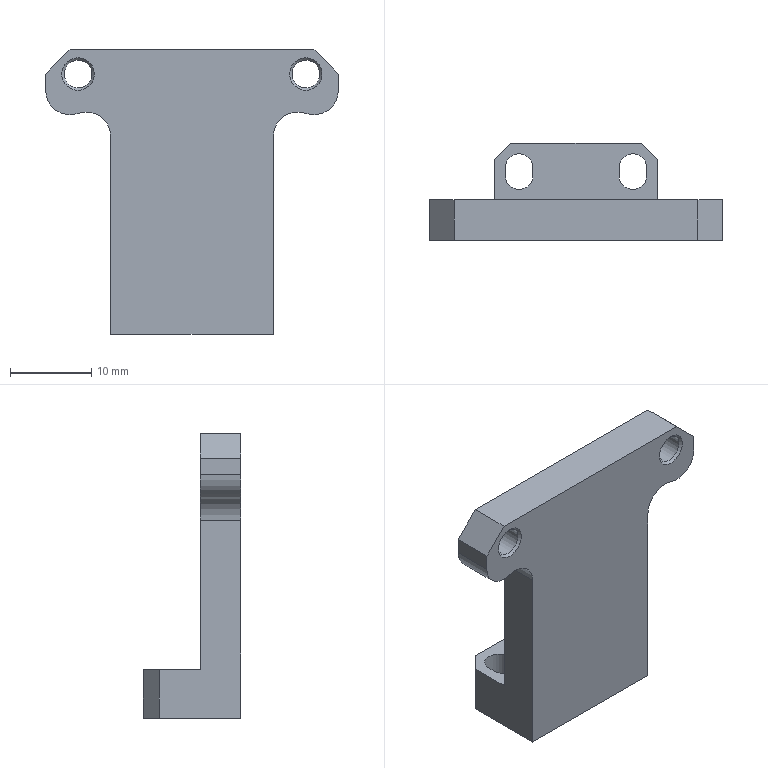Part | NX | features DATUM_CSYS 5, SKETCH 4, EXTRUDE 3, CHAMFER 2, OFFSET_REGION 2, SIMPLE HOLE 2, BLEND 1, HOLE PACKAGE 1 | 1 solid | 30 faces | box 36 x 12 x 35 mm | volume 4656 mm3 | plane 18 | cylinder 10 | cone 2 | commonest cylinder face diameters 3.4 x6 6 x4
STEP:
#1=CARTESIAN_POINT('',(23.3,9.,5.));
#2=VERTEX_POINT('',#1);
#3=CARTESIAN_POINT('',(23.3,8.,5.));
#4=VERTEX_POINT('',#3);
#5=CARTESIAN_POINT('',(23.3,9.,5.));
#6=DIRECTION('',(0.,-1.,0.));
#7=VECTOR('',#6,1000.);
#8=LINE('',#5,#7);
#9=EDGE_CURVE('',#2,#4,#8,.T.);
#10=ORIENTED_EDGE('',*,*,#9,.F.);
#11=CARTESIAN_POINT('',(26.7,9.,5.));
#12=VERTEX_POINT('',#11);
#13=CARTESIAN_POINT('',(25.,9.,5.));
#14=DIRECTION('',(0.,0.,1.));
#15=DIRECTION('',(0.,1.,0.));
#16=AXIS2_PLACEMENT_3D('',#13,#14,#15);
#17=CIRCLE('',#16,1.7);
#18=EDGE_CURVE('',#12,#2,#17,.T.);
#19=ORIENTED_EDGE('',*,*,#18,.F.);
#20=CARTESIAN_POINT('',(26.7,8.,5.));
#21=VERTEX_POINT('',#20);
#22=CARTESIAN_POINT('',(26.7,8.,5.));
#23=DIRECTION('',(0.,1.,0.));
#24=VECTOR('',#23,1000.);
#25=LINE('',#22,#24);
#26=EDGE_CURVE('',#21,#12,#25,.T.);
#27=ORIENTED_EDGE('',*,*,#26,.F.);
#28=CARTESIAN_POINT('',(25.,8.,5.));
#29=DIRECTION('',(0.,0.,1.));
#30=DIRECTION('',(0.,1.,0.));
#31=AXIS2_PLACEMENT_3D('',#28,#29,#30);
#32=CIRCLE('',#31,1.7);
#33=EDGE_CURVE('',#4,#21,#32,.T.);
#34=ORIENTED_EDGE('',*,*,#33,.F.);
#35=EDGE_LOOP('',(#10,#19,#27,#34));
#36=FACE_BOUND('',#35,.T.);
#37=CARTESIAN_POINT('',(26.,12.,5.));
#38=VERTEX_POINT('',#37);
#39=CARTESIAN_POINT('',(10.,12.,5.));
#40=VERTEX_POINT('',#39);
#41=CARTESIAN_POINT('',(36.,12.,5.));
#42=DIRECTION('',(-1.,0.,0.));
#43=VECTOR('',#42,1000.);
#44=LINE('',#41,#43);
#45=EDGE_CURVE('',#38,#40,#44,.T.);
#46=ORIENTED_EDGE('',*,*,#45,.T.);
#47=CARTESIAN_POINT('',(8.,10.,5.));
#48=VERTEX_POINT('',#47);
#49=CARTESIAN_POINT('',(8.,10.,5.));
#50=DIRECTION('',(0.7071,0.7071,0.));
#51=VECTOR('',#50,1000.);
#52=LINE('',#49,#51);
#53=EDGE_CURVE('',#40,#48,#52,.F.);
#54=ORIENTED_EDGE('',*,*,#53,.T.);
#55=CARTESIAN_POINT('',(8.,5.,5.));
#56=VERTEX_POINT('',#55);
#57=CARTESIAN_POINT('',(8.,12.,5.));
#58=DIRECTION('',(0.,-1.,0.));
#59=VECTOR('',#58,1000.);
#60=LINE('',#57,#59);
#61=EDGE_CURVE('',#48,#56,#60,.T.);
#62=ORIENTED_EDGE('',*,*,#61,.T.);
#63=CARTESIAN_POINT('',(28.,5.,5.));
#64=VERTEX_POINT('',#63);
#65=CARTESIAN_POINT('',(36.,5.,5.));
#66=DIRECTION('',(-1.,0.,0.));
#67=VECTOR('',#66,1000.);
#68=LINE('',#65,#67);
#69=EDGE_CURVE('',#64,#56,#68,.T.);
#70=ORIENTED_EDGE('',*,*,#69,.F.);
#71=CARTESIAN_POINT('',(28.,10.,5.));
#72=VERTEX_POINT('',#71);
#73=CARTESIAN_POINT('',(28.,12.,5.));
#74=DIRECTION('',(0.,1.,0.));
#75=VECTOR('',#74,1000.);
#76=LINE('',#73,#75);
#77=EDGE_CURVE('',#64,#72,#76,.T.);
#78=ORIENTED_EDGE('',*,*,#77,.T.);
#79=CARTESIAN_POINT('',(28.,10.,5.));
#80=DIRECTION('',(0.7071,-0.7071,0.));
#81=VECTOR('',#80,1000.);
#82=LINE('',#79,#81);
#83=EDGE_CURVE('',#72,#38,#82,.F.);
#84=ORIENTED_EDGE('',*,*,#83,.T.);
#85=EDGE_LOOP('',(#46,#54,#62,#70,#78,#84));
#86=FACE_BOUND('',#85,.T.);
#87=CARTESIAN_POINT('',(9.3,9.,5.));
#88=VERTEX_POINT('',#87);
#89=CARTESIAN_POINT('',(9.3,8.,5.));
#90=VERTEX_POINT('',#89);
#91=CARTESIAN_POINT('',(9.3,9.,5.));
#92=DIRECTION('',(0.,-1.,0.));
#93=VECTOR('',#92,1000.);
#94=LINE('',#91,#93);
#95=EDGE_CURVE('',#88,#90,#94,.T.);
#96=ORIENTED_EDGE('',*,*,#95,.F.);
#97=CARTESIAN_POINT('',(12.7,9.,5.));
#98=VERTEX_POINT('',#97);
#99=CARTESIAN_POINT('',(11.,9.,5.));
#100=DIRECTION('',(0.,0.,1.));
#101=DIRECTION('',(0.,1.,0.));
#102=AXIS2_PLACEMENT_3D('',#99,#100,#101);
#103=CIRCLE('',#102,1.7);
#104=EDGE_CURVE('',#98,#88,#103,.T.);
#105=ORIENTED_EDGE('',*,*,#104,.F.);
#106=CARTESIAN_POINT('',(12.7,8.,5.));
#107=VERTEX_POINT('',#106);
#108=CARTESIAN_POINT('',(12.7,8.,5.));
#109=DIRECTION('',(0.,1.,0.));
#110=VECTOR('',#109,1000.);
#111=LINE('',#108,#110);
#112=EDGE_CURVE('',#107,#98,#111,.T.);
#113=ORIENTED_EDGE('',*,*,#112,.F.);
#114=CARTESIAN_POINT('',(11.,8.,5.));
#115=DIRECTION('',(0.,0.,1.));
#116=DIRECTION('',(0.,1.,0.));
#117=AXIS2_PLACEMENT_3D('',#114,#115,#116);
#118=CIRCLE('',#117,1.7);
#119=EDGE_CURVE('',#90,#107,#118,.T.);
#120=ORIENTED_EDGE('',*,*,#119,.F.);
#121=EDGE_LOOP('',(#96,#105,#113,#120));
#122=FACE_BOUND('',#121,.T.);
#123=CARTESIAN_POINT('',(36.,12.,5.));
#124=DIRECTION('',(0.,0.,-1.));
#125=DIRECTION('',(0.,1.,0.));
#126=AXIS2_PLACEMENT_3D('',#123,#124,#125);
#127=PLANE('',#126);
#128=ADVANCED_FACE('',(#36,#86,#122),#127,.F.);
#129=CARTESIAN_POINT('',(26.,12.,-1.));
#130=VERTEX_POINT('',#129);
#131=CARTESIAN_POINT('',(10.,12.,-1.));
#132=VERTEX_POINT('',#131);
#133=CARTESIAN_POINT('',(36.,12.,-1.));
#134=DIRECTION('',(-1.,0.,0.));
#135=VECTOR('',#134,1000.);
#136=LINE('',#133,#135);
#137=EDGE_CURVE('',#130,#132,#136,.T.);
#138=ORIENTED_EDGE('',*,*,#137,.T.);
#139=CARTESIAN_POINT('',(10.,12.,0.));
#140=DIRECTION('',(0.,0.,1.));
#141=VECTOR('',#140,1000.);
#142=LINE('',#139,#141);
#143=EDGE_CURVE('',#132,#40,#142,.T.);
#144=ORIENTED_EDGE('',*,*,#143,.T.);
#145=ORIENTED_EDGE('',*,*,#45,.F.);
#146=CARTESIAN_POINT('',(26.,12.,0.));
#147=DIRECTION('',(0.,0.,-1.));
#148=VECTOR('',#147,1000.);
#149=LINE('',#146,#148);
#150=EDGE_CURVE('',#38,#130,#149,.T.);
#151=ORIENTED_EDGE('',*,*,#150,.T.);
#152=EDGE_LOOP('',(#138,#144,#145,#151));
#153=FACE_BOUND('',#152,.T.);
#154=CARTESIAN_POINT('',(36.,12.,0.));
#155=DIRECTION('',(0.,-1.,0.));
#156=DIRECTION('',(0.,0.,-1.));
#157=AXIS2_PLACEMENT_3D('',#154,#155,#156);
#158=PLANE('',#157);
#159=ADVANCED_FACE('',(#153),#158,.F.);
#160=CARTESIAN_POINT('',(0.,0.,31.));
#161=VERTEX_POINT('',#160);
#162=CARTESIAN_POINT('',(0.,0.,29.));
#163=VERTEX_POINT('',#162);
#164=CARTESIAN_POINT('',(0.,0.,34.));
#165=DIRECTION('',(0.,0.,-1.));
#166=VECTOR('',#165,1000.);
#167=LINE('',#164,#166);
#168=EDGE_CURVE('',#161,#163,#167,.T.);
#169=ORIENTED_EDGE('',*,*,#168,.F.);
#170=CARTESIAN_POINT('',(0.,5.,31.));
#171=VERTEX_POINT('',#170);
#172=CARTESIAN_POINT('',(0.,0.,31.));
#173=DIRECTION('',(0.,1.,0.));
#174=VECTOR('',#173,1000.);
#175=LINE('',#172,#174);
#176=EDGE_CURVE('',#161,#171,#175,.T.);
#177=ORIENTED_EDGE('',*,*,#176,.T.);
#178=CARTESIAN_POINT('',(0.,5.,29.));
#179=VERTEX_POINT('',#178);
#180=CARTESIAN_POINT('',(0.,5.,5.));
#181=DIRECTION('',(0.,0.,1.));
#182=VECTOR('',#181,1000.);
#183=LINE('',#180,#182);
#184=EDGE_CURVE('',#179,#171,#183,.T.);
#185=ORIENTED_EDGE('',*,*,#184,.F.);
#186=CARTESIAN_POINT('',(0.,0.,29.));
#187=DIRECTION('',(0.,1.,0.));
#188=VECTOR('',#187,1000.);
#189=LINE('',#186,#188);
#190=EDGE_CURVE('',#179,#163,#189,.F.);
#191=ORIENTED_EDGE('',*,*,#190,.T.);
#192=EDGE_LOOP('',(#169,#177,#185,#191));
#193=FACE_BOUND('',#192,.T.);
#194=CARTESIAN_POINT('',(0.,0.,0.));
#195=DIRECTION('',(1.,0.,0.));
#196=DIRECTION('',(0.,0.,-1.));
#197=AXIS2_PLACEMENT_3D('',#194,#195,#196);
#198=PLANE('',#197);
#199=ADVANCED_FACE('',(#193),#198,.F.);
#200=CARTESIAN_POINT('',(12.7,9.,-1.));
#201=VERTEX_POINT('',#200);
#202=CARTESIAN_POINT('',(9.3,9.,-1.));
#203=VERTEX_POINT('',#202);
#204=CARTESIAN_POINT('',(11.,9.,-1.));
#205=DIRECTION('',(0.,0.,1.));
#206=DIRECTION('',(1.,0.,0.));
#207=AXIS2_PLACEMENT_3D('',#204,#205,#206);
#208=CIRCLE('',#207,1.7);
#209=EDGE_CURVE('',#201,#203,#208,.T.);
#210=ORIENTED_EDGE('',*,*,#209,.T.);
#211=CARTESIAN_POINT('',(9.3,8.,-1.));
#212=VERTEX_POINT('',#211);
#213=CARTESIAN_POINT('',(9.3,5.,-1.));
#214=DIRECTION('',(0.,-1.,0.));
#215=VECTOR('',#214,1000.);
#216=LINE('',#213,#215);
#217=EDGE_CURVE('',#203,#212,#216,.T.);
#218=ORIENTED_EDGE('',*,*,#217,.T.);
#219=CARTESIAN_POINT('',(12.7,8.,-1.));
#220=VERTEX_POINT('',#219);
#221=CARTESIAN_POINT('',(11.,8.,-1.));
#222=DIRECTION('',(0.,0.,1.));
#223=DIRECTION('',(1.,0.,0.));
#224=AXIS2_PLACEMENT_3D('',#221,#222,#223);
#225=CIRCLE('',#224,1.7);
#226=EDGE_CURVE('',#212,#220,#225,.T.);
#227=ORIENTED_EDGE('',*,*,#226,.T.);
#228=CARTESIAN_POINT('',(12.7,5.,-1.));
#229=DIRECTION('',(0.,1.,0.));
#230=VECTOR('',#229,1000.);
#231=LINE('',#228,#230);
#232=EDGE_CURVE('',#220,#201,#231,.T.);
#233=ORIENTED_EDGE('',*,*,#232,.T.);
#234=EDGE_LOOP('',(#210,#218,#227,#233));
#235=FACE_BOUND('',#234,.T.);
#236=CARTESIAN_POINT('',(26.7,9.,-1.));
#237=VERTEX_POINT('',#236);
#238=CARTESIAN_POINT('',(23.3,9.,-1.));
#239=VERTEX_POINT('',#238);
#240=CARTESIAN_POINT('',(25.,9.,-1.));
#241=DIRECTION('',(0.,0.,1.));
#242=DIRECTION('',(1.,0.,0.));
#243=AXIS2_PLACEMENT_3D('',#240,#241,#242);
#244=CIRCLE('',#243,1.7);
#245=EDGE_CURVE('',#237,#239,#244,.T.);
#246=ORIENTED_EDGE('',*,*,#245,.T.);
#247=CARTESIAN_POINT('',(23.3,8.,-1.));
#248=VERTEX_POINT('',#247);
#249=CARTESIAN_POINT('',(23.3,5.,-1.));
#250=DIRECTION('',(0.,-1.,0.));
#251=VECTOR('',#250,1000.);
#252=LINE('',#249,#251);
#253=EDGE_CURVE('',#239,#248,#252,.T.);
#254=ORIENTED_EDGE('',*,*,#253,.T.);
#255=CARTESIAN_POINT('',(26.7,8.,-1.));
#256=VERTEX_POINT('',#255);
#257=CARTESIAN_POINT('',(25.,8.,-1.));
#258=DIRECTION('',(0.,0.,1.));
#259=DIRECTION('',(1.,0.,0.));
#260=AXIS2_PLACEMENT_3D('',#257,#258,#259);
#261=CIRCLE('',#260,1.7);
#262=EDGE_CURVE('',#248,#256,#261,.T.);
#263=ORIENTED_EDGE('',*,*,#262,.T.);
#264=CARTESIAN_POINT('',(26.7,5.,-1.));
#265=DIRECTION('',(0.,1.,0.));
#266=VECTOR('',#265,1000.);
#267=LINE('',#264,#266);
#268=EDGE_CURVE('',#256,#237,#267,.T.);
#269=ORIENTED_EDGE('',*,*,#268,.T.);
#270=EDGE_LOOP('',(#246,#254,#263,#269));
#271=FACE_BOUND('',#270,.T.);
#272=CARTESIAN_POINT('',(8.,0.,-1.));
#273=VERTEX_POINT('',#272);
#274=CARTESIAN_POINT('',(8.,10.,-1.));
#275=VERTEX_POINT('',#274);
#276=CARTESIAN_POINT('',(8.,5.,-1.));
#277=DIRECTION('',(0.,1.,0.));
#278=VECTOR('',#277,1000.);
#279=LINE('',#276,#278);
#280=EDGE_CURVE('',#273,#275,#279,.T.);
#281=ORIENTED_EDGE('',*,*,#280,.T.);
#282=CARTESIAN_POINT('',(8.,10.,-1.));
#283=DIRECTION('',(-0.7071,-0.7071,0.));
#284=VECTOR('',#283,1000.);
#285=LINE('',#282,#284);
#286=EDGE_CURVE('',#275,#132,#285,.F.);
#287=ORIENTED_EDGE('',*,*,#286,.T.);
#288=ORIENTED_EDGE('',*,*,#137,.F.);
#289=CARTESIAN_POINT('',(28.,10.,-1.));
#290=VERTEX_POINT('',#289);
#291=CARTESIAN_POINT('',(28.,10.,-1.));
#292=DIRECTION('',(-0.7071,0.7071,0.));
#293=VECTOR('',#292,1000.);
#294=LINE('',#291,#293);
#295=EDGE_CURVE('',#130,#290,#294,.F.);
#296=ORIENTED_EDGE('',*,*,#295,.T.);
#297=CARTESIAN_POINT('',(28.,0.,-1.));
#298=VERTEX_POINT('',#297);
#299=CARTESIAN_POINT('',(28.,-38.,-1.));
#300=DIRECTION('',(0.,1.,0.));
#301=VECTOR('',#300,1000.);
#302=LINE('',#299,#301);
#303=EDGE_CURVE('',#298,#290,#302,.T.);
#304=ORIENTED_EDGE('',*,*,#303,.F.);
#305=CARTESIAN_POINT('',(36.,0.,-1.));
#306=DIRECTION('',(-1.,0.,0.));
#307=VECTOR('',#306,1000.);
#308=LINE('',#305,#307);
#309=EDGE_CURVE('',#298,#273,#308,.T.);
#310=ORIENTED_EDGE('',*,*,#309,.T.);
#311=EDGE_LOOP('',(#281,#287,#288,#296,#304,#310));
#312=FACE_BOUND('',#311,.T.);
#313=CARTESIAN_POINT('',(36.,5.,-1.));
#314=DIRECTION('',(0.,0.,1.));
#315=DIRECTION('',(1.,0.,0.));
#316=AXIS2_PLACEMENT_3D('',#313,#314,#315);
#317=PLANE('',#316);
#318=ADVANCED_FACE('',(#235,#271,#312),#317,.F.);
#319=CARTESIAN_POINT('',(36.,5.,29.));
#320=VERTEX_POINT('',#319);
#321=CARTESIAN_POINT('',(36.,5.,31.));
#322=VERTEX_POINT('',#321);
#323=CARTESIAN_POINT('',(36.,5.,5.));
#324=DIRECTION('',(0.,0.,1.));
#325=VECTOR('',#324,1000.);
#326=LINE('',#323,#325);
#327=EDGE_CURVE('',#320,#322,#326,.T.);
#328=ORIENTED_EDGE('',*,*,#327,.T.);
#329=CARTESIAN_POINT('',(36.,0.,31.));
#330=VERTEX_POINT('',#329);
#331=CARTESIAN_POINT('',(36.,0.,31.));
#332=DIRECTION('',(0.,-1.,0.));
#333=VECTOR('',#332,1000.);
#334=LINE('',#331,#333);
#335=EDGE_CURVE('',#322,#330,#334,.T.);
#336=ORIENTED_EDGE('',*,*,#335,.T.);
#337=CARTESIAN_POINT('',(36.,0.,29.));
#338=VERTEX_POINT('',#337);
#339=CARTESIAN_POINT('',(36.,0.,5.));
#340=DIRECTION('',(0.,0.,-1.));
#341=VECTOR('',#340,1000.);
#342=LINE('',#339,#341);
#343=EDGE_CURVE('',#330,#338,#342,.T.);
#344=ORIENTED_EDGE('',*,*,#343,.T.);
#345=CARTESIAN_POINT('',(36.,5.,29.));
#346=DIRECTION('',(0.,1.,0.));
#347=VECTOR('',#346,1000.);
#348=LINE('',#345,#347);
#349=EDGE_CURVE('',#338,#320,#348,.T.);
#350=ORIENTED_EDGE('',*,*,#349,.T.);
#351=EDGE_LOOP('',(#328,#336,#344,#350));
#352=FACE_BOUND('',#351,.T.);
#353=CARTESIAN_POINT('',(36.,0.,0.));
#354=DIRECTION('',(1.,0.,0.));
#355=DIRECTION('',(0.,0.,-1.));
#356=AXIS2_PLACEMENT_3D('',#353,#354,#355);
#357=PLANE('',#356);
#358=ADVANCED_FACE('',(#352),#357,.T.);
#359=CARTESIAN_POINT('',(3.995,5.,29.3));
#360=VERTEX_POINT('',#359);
#361=CARTESIAN_POINT('',(3.995,5.,31.));
#362=DIRECTION('',(0.,-1.,0.));
#363=DIRECTION('',(0.,0.,-1.));
#364=AXIS2_PLACEMENT_3D('',#361,#362,#363);
#365=CIRCLE('',#364,1.7);
#366=EDGE_CURVE('',#360,#360,#365,.T.);
#367=ORIENTED_EDGE('',*,*,#366,.T.);
#368=EDGE_LOOP('',(#367));
#369=FACE_BOUND('',#368,.T.);
#370=CARTESIAN_POINT('',(32.,5.,29.3));
#371=VERTEX_POINT('',#370);
#372=CARTESIAN_POINT('',(32.,5.,31.));
#373=DIRECTION('',(0.,-1.,0.));
#374=DIRECTION('',(0.,0.,-1.));
#375=AXIS2_PLACEMENT_3D('',#372,#373,#374);
#376=CIRCLE('',#375,1.7);
#377=EDGE_CURVE('',#371,#371,#376,.T.);
#378=ORIENTED_EDGE('',*,*,#377,.T.);
#379=EDGE_LOOP('',(#378));
#380=FACE_BOUND('',#379,.T.);
#381=CARTESIAN_POINT('',(33.,5.,34.));
#382=VERTEX_POINT('',#381);
#383=CARTESIAN_POINT('',(3.,5.,34.));
#384=VERTEX_POINT('',#383);
#385=CARTESIAN_POINT('',(36.,5.,34.));
#386=DIRECTION('',(-1.,0.,0.));
#387=VECTOR('',#386,1000.);
#388=LINE('',#385,#387);
#389=EDGE_CURVE('',#382,#384,#388,.T.);
#390=ORIENTED_EDGE('',*,*,#389,.F.);
#391=CARTESIAN_POINT('',(36.,5.,31.));
#392=DIRECTION('',(0.7071,0.,-0.7071));
#393=VECTOR('',#392,1000.);
#394=LINE('',#391,#393);
#395=EDGE_CURVE('',#382,#322,#394,.T.);
#396=ORIENTED_EDGE('',*,*,#395,.T.);
#397=ORIENTED_EDGE('',*,*,#327,.F.);
#398=CARTESIAN_POINT('',(32.,5.,26.172));
#399=VERTEX_POINT('',#398);
#400=CARTESIAN_POINT('',(33.,5.,29.));
#401=DIRECTION('',(0.,-1.,0.));
#402=DIRECTION('',(0.,0.,-1.));
#403=AXIS2_PLACEMENT_3D('',#400,#401,#402);
#404=CIRCLE('',#403,3.);
#405=EDGE_CURVE('',#320,#399,#404,.F.);
#406=ORIENTED_EDGE('',*,*,#405,.T.);
#407=CARTESIAN_POINT('',(28.,5.,23.343));
#408=VERTEX_POINT('',#407);
#409=CARTESIAN_POINT('',(31.,5.,23.343));
#410=DIRECTION('',(0.,-1.,0.));
#411=DIRECTION('',(0.,0.,-1.));
#412=AXIS2_PLACEMENT_3D('',#409,#410,#411);
#413=CIRCLE('',#412,3.);
#414=EDGE_CURVE('',#399,#408,#413,.T.);
#415=ORIENTED_EDGE('',*,*,#414,.T.);
#416=CARTESIAN_POINT('',(28.,5.,5.));
#417=DIRECTION('',(0.,0.,-1.));
#418=VECTOR('',#417,1000.);
#419=LINE('',#416,#418);
#420=EDGE_CURVE('',#408,#64,#419,.T.);
#421=ORIENTED_EDGE('',*,*,#420,.T.);
#422=ORIENTED_EDGE('',*,*,#69,.T.);
#423=CARTESIAN_POINT('',(8.,5.,23.343));
#424=VERTEX_POINT('',#423);
#425=CARTESIAN_POINT('',(8.,5.,5.));
#426=DIRECTION('',(0.,0.,1.));
#427=VECTOR('',#426,1000.);
#428=LINE('',#425,#427);
#429=EDGE_CURVE('',#56,#424,#428,.T.);
#430=ORIENTED_EDGE('',*,*,#429,.T.);
#431=CARTESIAN_POINT('',(4.,5.,26.172));
#432=VERTEX_POINT('',#431);
#433=CARTESIAN_POINT('',(5.,5.,23.343));
#434=DIRECTION('',(0.,-1.,0.));
#435=DIRECTION('',(0.,0.,-1.));
#436=AXIS2_PLACEMENT_3D('',#433,#434,#435);
#437=CIRCLE('',#436,3.);
#438=EDGE_CURVE('',#424,#432,#437,.T.);
#439=ORIENTED_EDGE('',*,*,#438,.T.);
#440=CARTESIAN_POINT('',(3.,5.,29.));
#441=DIRECTION('',(0.,-1.,0.));
#442=DIRECTION('',(0.,0.,-1.));
#443=AXIS2_PLACEMENT_3D('',#440,#441,#442);
#444=CIRCLE('',#443,3.);
#445=EDGE_CURVE('',#432,#179,#444,.F.);
#446=ORIENTED_EDGE('',*,*,#445,.T.);
#447=ORIENTED_EDGE('',*,*,#184,.T.);
#448=CARTESIAN_POINT('',(3.,5.,34.));
#449=DIRECTION('',(-0.7071,0.,-0.7071));
#450=VECTOR('',#449,1000.);
#451=LINE('',#448,#450);
#452=EDGE_CURVE('',#171,#384,#451,.F.);
#453=ORIENTED_EDGE('',*,*,#452,.T.);
#454=EDGE_LOOP('',(#390,#396,#397,#406,#415,#421,#422,#430,#439,#446,#447,#453));
#455=FACE_BOUND('',#454,.T.);
#456=CARTESIAN_POINT('',(36.,5.,5.));
#457=DIRECTION('',(0.,-1.,0.));
#458=DIRECTION('',(0.,0.,-1.));
#459=AXIS2_PLACEMENT_3D('',#456,#457,#458);
#460=PLANE('',#459);
#461=ADVANCED_FACE('',(#369,#380,#455),#460,.F.);
#462=CARTESIAN_POINT('',(33.,0.,34.));
#463=VERTEX_POINT('',#462);
#464=CARTESIAN_POINT('',(3.,0.,34.));
#465=VERTEX_POINT('',#464);
#466=CARTESIAN_POINT('',(36.,0.,34.));
#467=DIRECTION('',(-1.,0.,0.));
#468=VECTOR('',#467,1000.);
#469=LINE('',#466,#468);
#470=EDGE_CURVE('',#463,#465,#469,.T.);
#471=ORIENTED_EDGE('',*,*,#470,.F.);
#472=CARTESIAN_POINT('',(33.,5.,34.));
#473=DIRECTION('',(0.,1.,0.));
#474=VECTOR('',#473,1000.);
#475=LINE('',#472,#474);
#476=EDGE_CURVE('',#463,#382,#475,.T.);
#477=ORIENTED_EDGE('',*,*,#476,.T.);
#478=ORIENTED_EDGE('',*,*,#389,.T.);
#479=CARTESIAN_POINT('',(3.,5.,34.));
#480=DIRECTION('',(0.,-1.,0.));
#481=VECTOR('',#480,1000.);
#482=LINE('',#479,#481);
#483=EDGE_CURVE('',#384,#465,#482,.T.);
#484=ORIENTED_EDGE('',*,*,#483,.T.);
#485=EDGE_LOOP('',(#471,#477,#478,#484));
#486=FACE_BOUND('',#485,.T.);
#487=CARTESIAN_POINT('',(36.,5.,34.));
#488=DIRECTION('',(0.,0.,-1.));
#489=DIRECTION('',(-1.,0.,0.));
#490=AXIS2_PLACEMENT_3D('',#487,#488,#489);
#491=PLANE('',#490);
#492=ADVANCED_FACE('',(#486),#491,.F.);
#493=CARTESIAN_POINT('',(3.995,0.,33.));
#494=VERTEX_POINT('',#493);
#495=CARTESIAN_POINT('',(3.995,0.,31.));
#496=DIRECTION('',(0.,1.,0.));
#497=DIRECTION('',(0.,0.,1.));
#498=AXIS2_PLACEMENT_3D('',#495,#496,#497);
#499=CIRCLE('',#498,2.);
#500=EDGE_CURVE('',#494,#494,#499,.T.);
#501=ORIENTED_EDGE('',*,*,#500,.T.);
#502=EDGE_LOOP('',(#501));
#503=FACE_BOUND('',#502,.T.);
#504=CARTESIAN_POINT('',(32.,0.,33.));
#505=VERTEX_POINT('',#504);
#506=CARTESIAN_POINT('',(32.,0.,31.));
#507=DIRECTION('',(0.,1.,0.));
#508=DIRECTION('',(0.,0.,1.));
#509=AXIS2_PLACEMENT_3D('',#506,#507,#508);
#510=CIRCLE('',#509,2.);
#511=EDGE_CURVE('',#505,#505,#510,.T.);
#512=ORIENTED_EDGE('',*,*,#511,.T.);
#513=EDGE_LOOP('',(#512));
#514=FACE_BOUND('',#513,.T.);
#515=ORIENTED_EDGE('',*,*,#343,.F.);
#516=CARTESIAN_POINT('',(36.,0.,31.));
#517=DIRECTION('',(-0.7071,0.,0.7071));
#518=VECTOR('',#517,1000.);
#519=LINE('',#516,#518);
#520=EDGE_CURVE('',#330,#463,#519,.T.);
#521=ORIENTED_EDGE('',*,*,#520,.T.);
#522=ORIENTED_EDGE('',*,*,#470,.T.);
#523=CARTESIAN_POINT('',(3.,0.,34.));
#524=DIRECTION('',(0.7071,0.,0.7071));
#525=VECTOR('',#524,1000.);
#526=LINE('',#523,#525);
#527=EDGE_CURVE('',#465,#161,#526,.F.);
#528=ORIENTED_EDGE('',*,*,#527,.T.);
#529=ORIENTED_EDGE('',*,*,#168,.T.);
#530=CARTESIAN_POINT('',(4.,0.,26.172));
#531=VERTEX_POINT('',#530);
#532=CARTESIAN_POINT('',(3.,0.,29.));
#533=DIRECTION('',(0.,1.,0.));
#534=DIRECTION('',(0.,0.,1.));
#535=AXIS2_PLACEMENT_3D('',#532,#533,#534);
#536=CIRCLE('',#535,3.);
#537=EDGE_CURVE('',#163,#531,#536,.F.);
#538=ORIENTED_EDGE('',*,*,#537,.T.);
#539=CARTESIAN_POINT('',(8.,0.,23.343));
#540=VERTEX_POINT('',#539);
#541=CARTESIAN_POINT('',(5.,0.,23.343));
#542=DIRECTION('',(0.,1.,0.));
#543=DIRECTION('',(0.,0.,1.));
#544=AXIS2_PLACEMENT_3D('',#541,#542,#543);
#545=CIRCLE('',#544,3.);
#546=EDGE_CURVE('',#531,#540,#545,.T.);
#547=ORIENTED_EDGE('',*,*,#546,.T.);
#548=CARTESIAN_POINT('',(8.,0.,34.));
#549=DIRECTION('',(0.,0.,-1.));
#550=VECTOR('',#549,1000.);
#551=LINE('',#548,#550);
#552=EDGE_CURVE('',#540,#273,#551,.T.);
#553=ORIENTED_EDGE('',*,*,#552,.T.);
#554=ORIENTED_EDGE('',*,*,#309,.F.);
#555=CARTESIAN_POINT('',(28.,0.,23.343));
#556=VERTEX_POINT('',#555);
#557=CARTESIAN_POINT('',(28.,0.,34.));
#558=DIRECTION('',(0.,0.,1.));
#559=VECTOR('',#558,1000.);
#560=LINE('',#557,#559);
#561=EDGE_CURVE('',#298,#556,#560,.T.);
#562=ORIENTED_EDGE('',*,*,#561,.T.);
#563=CARTESIAN_POINT('',(32.,0.,26.172));
#564=VERTEX_POINT('',#563);
#565=CARTESIAN_POINT('',(31.,0.,23.343));
#566=DIRECTION('',(0.,1.,0.));
#567=DIRECTION('',(0.,0.,1.));
#568=AXIS2_PLACEMENT_3D('',#565,#566,#567);
#569=CIRCLE('',#568,3.);
#570=EDGE_CURVE('',#556,#564,#569,.T.);
#571=ORIENTED_EDGE('',*,*,#570,.T.);
#572=CARTESIAN_POINT('',(33.,0.,29.));
#573=DIRECTION('',(0.,1.,0.));
#574=DIRECTION('',(0.,0.,1.));
#575=AXIS2_PLACEMENT_3D('',#572,#573,#574);
#576=CIRCLE('',#575,3.);
#577=EDGE_CURVE('',#564,#338,#576,.F.);
#578=ORIENTED_EDGE('',*,*,#577,.T.);
#579=EDGE_LOOP('',(#515,#521,#522,#528,#529,#538,#547,#553,#554,#562,#571,#578));
#580=FACE_BOUND('',#579,.T.);
#581=CARTESIAN_POINT('',(36.,0.,34.));
#582=DIRECTION('',(0.,1.,0.));
#583=DIRECTION('',(0.,0.,1.));
#584=AXIS2_PLACEMENT_3D('',#581,#582,#583);
#585=PLANE('',#584);
#586=ADVANCED_FACE('',(#503,#514,#580),#585,.F.);
#587=CARTESIAN_POINT('',(32.,0.3,32.7));
#588=VERTEX_POINT('',#587);
#589=CARTESIAN_POINT('',(32.,0.3,31.));
#590=DIRECTION('',(0.,1.,0.));
#591=DIRECTION('',(0.,0.,1.));
#592=AXIS2_PLACEMENT_3D('',#589,#590,#591);
#593=CIRCLE('',#592,1.7);
#594=EDGE_CURVE('',#588,#588,#593,.F.);
#595=ORIENTED_EDGE('',*,*,#594,.T.);
#596=EDGE_LOOP('',(#595));
#597=FACE_BOUND('',#596,.T.);
#598=ORIENTED_EDGE('',*,*,#377,.F.);
#599=EDGE_LOOP('',(#598));
#600=FACE_BOUND('',#599,.T.);
#601=CARTESIAN_POINT('',(32.,5.,31.));
#602=DIRECTION('',(0.,-1.,0.));
#603=DIRECTION('',(0.,0.,-1.));
#604=AXIS2_PLACEMENT_3D('',#601,#602,#603);
#605=CYLINDRICAL_SURFACE('',#604,1.7);
#606=ADVANCED_FACE('',(#597,#600),#605,.F.);
#607=ORIENTED_EDGE('',*,*,#594,.F.);
#608=EDGE_LOOP('',(#607));
#609=FACE_BOUND('',#608,.T.);
#610=ORIENTED_EDGE('',*,*,#511,.F.);
#611=EDGE_LOOP('',(#610));
#612=FACE_BOUND('',#611,.T.);
#613=CARTESIAN_POINT('',(32.,0.,31.));
#614=DIRECTION('',(0.,-1.,0.));
#615=DIRECTION('',(0.,0.,-1.));
#616=AXIS2_PLACEMENT_3D('',#613,#614,#615);
#617=CONICAL_SURFACE('',#616,2.,0.7854);
#618=ADVANCED_FACE('',(#609,#612),#617,.F.);
#619=CARTESIAN_POINT('',(3.995,0.3,32.7));
#620=VERTEX_POINT('',#619);
#621=CARTESIAN_POINT('',(3.995,0.3,31.));
#622=DIRECTION('',(0.,1.,0.));
#623=DIRECTION('',(0.,0.,1.));
#624=AXIS2_PLACEMENT_3D('',#621,#622,#623);
#625=CIRCLE('',#624,1.7);
#626=EDGE_CURVE('',#620,#620,#625,.F.);
#627=ORIENTED_EDGE('',*,*,#626,.T.);
#628=EDGE_LOOP('',(#627));
#629=FACE_BOUND('',#628,.T.);
#630=ORIENTED_EDGE('',*,*,#366,.F.);
#631=EDGE_LOOP('',(#630));
#632=FACE_BOUND('',#631,.T.);
#633=CARTESIAN_POINT('',(3.995,5.,31.));
#634=DIRECTION('',(0.,-1.,0.));
#635=DIRECTION('',(0.,0.,-1.));
#636=AXIS2_PLACEMENT_3D('',#633,#634,#635);
#637=CYLINDRICAL_SURFACE('',#636,1.7);
#638=ADVANCED_FACE('',(#629,#632),#637,.F.);
#639=ORIENTED_EDGE('',*,*,#626,.F.);
#640=EDGE_LOOP('',(#639));
#641=FACE_BOUND('',#640,.T.);
#642=ORIENTED_EDGE('',*,*,#500,.F.);
#643=EDGE_LOOP('',(#642));
#644=FACE_BOUND('',#643,.T.);
#645=CARTESIAN_POINT('',(3.995,0.,31.));
#646=DIRECTION('',(0.,-1.,0.));
#647=DIRECTION('',(0.,0.,-1.));
#648=AXIS2_PLACEMENT_3D('',#645,#646,#647);
#649=CONICAL_SURFACE('',#648,2.,0.7854);
#650=ADVANCED_FACE('',(#641,#644),#649,.F.);
#651=ORIENTED_EDGE('',*,*,#303,.T.);
#652=CARTESIAN_POINT('',(28.,10.,-1.));
#653=DIRECTION('',(0.,0.,1.));
#654=VECTOR('',#653,1000.);
#655=LINE('',#652,#654);
#656=EDGE_CURVE('',#290,#72,#655,.T.);
#657=ORIENTED_EDGE('',*,*,#656,.T.);
#658=ORIENTED_EDGE('',*,*,#77,.F.);
#659=ORIENTED_EDGE('',*,*,#420,.F.);
#660=CARTESIAN_POINT('',(28.,2.5,23.343));
#661=DIRECTION('',(0.,1.,0.));
#662=VECTOR('',#661,1000.);
#663=LINE('',#660,#662);
#664=EDGE_CURVE('',#408,#556,#663,.F.);
#665=ORIENTED_EDGE('',*,*,#664,.T.);
#666=ORIENTED_EDGE('',*,*,#561,.F.);
#667=EDGE_LOOP('',(#651,#657,#658,#659,#665,#666));
#668=FACE_BOUND('',#667,.T.);
#669=CARTESIAN_POINT('',(28.,-38.,-1.));
#670=DIRECTION('',(-1.,0.,0.));
#671=DIRECTION('',(0.,0.,1.));
#672=AXIS2_PLACEMENT_3D('',#669,#670,#671);
#673=PLANE('',#672);
#674=ADVANCED_FACE('',(#668),#673,.F.);
#675=ORIENTED_EDGE('',*,*,#61,.F.);
#676=CARTESIAN_POINT('',(8.,10.,26.));
#677=DIRECTION('',(0.,0.,-1.));
#678=VECTOR('',#677,1000.);
#679=LINE('',#676,#678);
#680=EDGE_CURVE('',#48,#275,#679,.T.);
#681=ORIENTED_EDGE('',*,*,#680,.T.);
#682=ORIENTED_EDGE('',*,*,#280,.F.);
#683=ORIENTED_EDGE('',*,*,#552,.F.);
#684=CARTESIAN_POINT('',(8.,2.5,23.343));
#685=DIRECTION('',(0.,1.,0.));
#686=VECTOR('',#685,1000.);
#687=LINE('',#684,#686);
#688=EDGE_CURVE('',#540,#424,#687,.T.);
#689=ORIENTED_EDGE('',*,*,#688,.T.);
#690=ORIENTED_EDGE('',*,*,#429,.F.);
#691=EDGE_LOOP('',(#675,#681,#682,#683,#689,#690));
#692=FACE_BOUND('',#691,.T.);
#693=CARTESIAN_POINT('',(8.,-38.,26.));
#694=DIRECTION('',(1.,0.,0.));
#695=DIRECTION('',(0.,0.,-1.));
#696=AXIS2_PLACEMENT_3D('',#693,#694,#695);
#697=PLANE('',#696);
#698=ADVANCED_FACE('',(#692),#697,.F.);
#699=ORIENTED_EDGE('',*,*,#688,.F.);
#700=ORIENTED_EDGE('',*,*,#546,.F.);
#701=CARTESIAN_POINT('',(4.,2.5,26.172));
#702=DIRECTION('',(0.,1.,0.));
#703=VECTOR('',#702,1000.);
#704=LINE('',#701,#703);
#705=EDGE_CURVE('',#432,#531,#704,.F.);
#706=ORIENTED_EDGE('',*,*,#705,.F.);
#707=ORIENTED_EDGE('',*,*,#438,.F.);
#708=EDGE_LOOP('',(#699,#700,#706,#707));
#709=FACE_BOUND('',#708,.T.);
#710=CARTESIAN_POINT('',(5.,-38.,23.343));
#711=DIRECTION('',(0.,1.,0.));
#712=DIRECTION('',(0.,0.,1.));
#713=AXIS2_PLACEMENT_3D('',#710,#711,#712);
#714=CYLINDRICAL_SURFACE('',#713,3.);
#715=ADVANCED_FACE('',(#709),#714,.F.);
#716=ORIENTED_EDGE('',*,*,#537,.F.);
#717=ORIENTED_EDGE('',*,*,#190,.F.);
#718=ORIENTED_EDGE('',*,*,#445,.F.);
#719=ORIENTED_EDGE('',*,*,#705,.T.);
#720=EDGE_LOOP('',(#716,#717,#718,#719));
#721=FACE_BOUND('',#720,.T.);
#722=CARTESIAN_POINT('',(3.,-38.,29.));
#723=DIRECTION('',(0.,1.,0.));
#724=DIRECTION('',(0.,0.,1.));
#725=AXIS2_PLACEMENT_3D('',#722,#723,#724);
#726=CYLINDRICAL_SURFACE('',#725,3.);
#727=ADVANCED_FACE('',(#721),#726,.T.);
#728=CARTESIAN_POINT('',(32.,2.5,26.172));
#729=DIRECTION('',(0.,1.,0.));
#730=VECTOR('',#729,1000.);
#731=LINE('',#728,#730);
#732=EDGE_CURVE('',#399,#564,#731,.F.);
#733=ORIENTED_EDGE('',*,*,#732,.F.);
#734=ORIENTED_EDGE('',*,*,#405,.F.);
#735=ORIENTED_EDGE('',*,*,#349,.F.);
#736=ORIENTED_EDGE('',*,*,#577,.F.);
#737=EDGE_LOOP('',(#733,#734,#735,#736));
#738=FACE_BOUND('',#737,.T.);
#739=CARTESIAN_POINT('',(33.,0.,29.));
#740=DIRECTION('',(0.,-1.,0.));
#741=DIRECTION('',(0.,0.,-1.));
#742=AXIS2_PLACEMENT_3D('',#739,#740,#741);
#743=CYLINDRICAL_SURFACE('',#742,3.);
#744=ADVANCED_FACE('',(#738),#743,.T.);
#745=ORIENTED_EDGE('',*,*,#414,.F.);
#746=ORIENTED_EDGE('',*,*,#732,.T.);
#747=ORIENTED_EDGE('',*,*,#570,.F.);
#748=ORIENTED_EDGE('',*,*,#664,.F.);
#749=EDGE_LOOP('',(#745,#746,#747,#748));
#750=FACE_BOUND('',#749,.T.);
#751=CARTESIAN_POINT('',(31.,-38.,23.343));
#752=DIRECTION('',(0.,1.,0.));
#753=DIRECTION('',(0.,0.,1.));
#754=AXIS2_PLACEMENT_3D('',#751,#752,#753);
#755=CYLINDRICAL_SURFACE('',#754,3.);
#756=ADVANCED_FACE('',(#750),#755,.F.);
#757=CARTESIAN_POINT('',(23.3,9.,-45.));
#758=DIRECTION('',(0.,0.,1.));
#759=VECTOR('',#758,1000.);
#760=LINE('',#757,#759);
#761=EDGE_CURVE('',#2,#239,#760,.F.);
#762=ORIENTED_EDGE('',*,*,#761,.F.);
#763=ORIENTED_EDGE('',*,*,#9,.T.);
#764=CARTESIAN_POINT('',(23.3,8.,-45.));
#765=DIRECTION('',(0.,0.,1.));
#766=VECTOR('',#765,1000.);
#767=LINE('',#764,#766);
#768=EDGE_CURVE('',#4,#248,#767,.F.);
#769=ORIENTED_EDGE('',*,*,#768,.T.);
#770=ORIENTED_EDGE('',*,*,#253,.F.);
#771=EDGE_LOOP('',(#762,#763,#769,#770));
#772=FACE_BOUND('',#771,.T.);
#773=CARTESIAN_POINT('',(23.3,9.,-45.));
#774=DIRECTION('',(-1.,0.,0.));
#775=DIRECTION('',(0.,0.,1.));
#776=AXIS2_PLACEMENT_3D('',#773,#774,#775);
#777=PLANE('',#776);
#778=ADVANCED_FACE('',(#772),#777,.F.);
#779=CARTESIAN_POINT('',(26.7,8.,-45.));
#780=DIRECTION('',(0.,0.,1.));
#781=VECTOR('',#780,1000.);
#782=LINE('',#779,#781);
#783=EDGE_CURVE('',#21,#256,#782,.F.);
#784=ORIENTED_EDGE('',*,*,#783,.F.);
#785=ORIENTED_EDGE('',*,*,#26,.T.);
#786=CARTESIAN_POINT('',(26.7,9.,-45.));
#787=DIRECTION('',(0.,0.,1.));
#788=VECTOR('',#787,1000.);
#789=LINE('',#786,#788);
#790=EDGE_CURVE('',#12,#237,#789,.F.);
#791=ORIENTED_EDGE('',*,*,#790,.T.);
#792=ORIENTED_EDGE('',*,*,#268,.F.);
#793=EDGE_LOOP('',(#784,#785,#791,#792));
#794=FACE_BOUND('',#793,.T.);
#795=CARTESIAN_POINT('',(26.7,8.,-45.));
#796=DIRECTION('',(1.,0.,0.));
#797=DIRECTION('',(0.,0.,-1.));
#798=AXIS2_PLACEMENT_3D('',#795,#796,#797);
#799=PLANE('',#798);
#800=ADVANCED_FACE('',(#794),#799,.F.);
#801=ORIENTED_EDGE('',*,*,#768,.F.);
#802=ORIENTED_EDGE('',*,*,#33,.T.);
#803=ORIENTED_EDGE('',*,*,#783,.T.);
#804=ORIENTED_EDGE('',*,*,#262,.F.);
#805=EDGE_LOOP('',(#801,#802,#803,#804));
#806=FACE_BOUND('',#805,.T.);
#807=CARTESIAN_POINT('',(25.,8.,-45.));
#808=DIRECTION('',(0.,0.,1.));
#809=DIRECTION('',(0.,-1.,0.));
#810=AXIS2_PLACEMENT_3D('',#807,#808,#809);
#811=CYLINDRICAL_SURFACE('',#810,1.7);
#812=ADVANCED_FACE('',(#806),#811,.F.);
#813=ORIENTED_EDGE('',*,*,#790,.F.);
#814=ORIENTED_EDGE('',*,*,#18,.T.);
#815=ORIENTED_EDGE('',*,*,#761,.T.);
#816=ORIENTED_EDGE('',*,*,#245,.F.);
#817=EDGE_LOOP('',(#813,#814,#815,#816));
#818=FACE_BOUND('',#817,.T.);
#819=CARTESIAN_POINT('',(25.,9.,-45.));
#820=DIRECTION('',(0.,0.,1.));
#821=DIRECTION('',(0.,-1.,0.));
#822=AXIS2_PLACEMENT_3D('',#819,#820,#821);
#823=CYLINDRICAL_SURFACE('',#822,1.7);
#824=ADVANCED_FACE('',(#818),#823,.F.);
#825=CARTESIAN_POINT('',(9.3,9.,-45.));
#826=DIRECTION('',(0.,0.,1.));
#827=VECTOR('',#826,1000.);
#828=LINE('',#825,#827);
#829=EDGE_CURVE('',#88,#203,#828,.F.);
#830=ORIENTED_EDGE('',*,*,#829,.F.);
#831=ORIENTED_EDGE('',*,*,#95,.T.);
#832=CARTESIAN_POINT('',(9.3,8.,-45.));
#833=DIRECTION('',(0.,0.,1.));
#834=VECTOR('',#833,1000.);
#835=LINE('',#832,#834);
#836=EDGE_CURVE('',#90,#212,#835,.F.);
#837=ORIENTED_EDGE('',*,*,#836,.T.);
#838=ORIENTED_EDGE('',*,*,#217,.F.);
#839=EDGE_LOOP('',(#830,#831,#837,#838));
#840=FACE_BOUND('',#839,.T.);
#841=CARTESIAN_POINT('',(9.3,9.,-45.));
#842=DIRECTION('',(-1.,0.,0.));
#843=DIRECTION('',(0.,0.,1.));
#844=AXIS2_PLACEMENT_3D('',#841,#842,#843);
#845=PLANE('',#844);
#846=ADVANCED_FACE('',(#840),#845,.F.);
#847=ORIENTED_EDGE('',*,*,#836,.F.);
#848=ORIENTED_EDGE('',*,*,#119,.T.);
#849=CARTESIAN_POINT('',(12.7,8.,-45.));
#850=DIRECTION('',(0.,0.,1.));
#851=VECTOR('',#850,1000.);
#852=LINE('',#849,#851);
#853=EDGE_CURVE('',#107,#220,#852,.F.);
#854=ORIENTED_EDGE('',*,*,#853,.T.);
#855=ORIENTED_EDGE('',*,*,#226,.F.);
#856=EDGE_LOOP('',(#847,#848,#854,#855));
#857=FACE_BOUND('',#856,.T.);
#858=CARTESIAN_POINT('',(11.,8.,-45.));
#859=DIRECTION('',(0.,0.,1.));
#860=DIRECTION('',(0.,-1.,0.));
#861=AXIS2_PLACEMENT_3D('',#858,#859,#860);
#862=CYLINDRICAL_SURFACE('',#861,1.7);
#863=ADVANCED_FACE('',(#857),#862,.F.);
#864=ORIENTED_EDGE('',*,*,#853,.F.);
#865=ORIENTED_EDGE('',*,*,#112,.T.);
#866=CARTESIAN_POINT('',(12.7,9.,-45.));
#867=DIRECTION('',(0.,0.,1.));
#868=VECTOR('',#867,1000.);
#869=LINE('',#866,#868);
#870=EDGE_CURVE('',#98,#201,#869,.F.);
#871=ORIENTED_EDGE('',*,*,#870,.T.);
#872=ORIENTED_EDGE('',*,*,#232,.F.);
#873=EDGE_LOOP('',(#864,#865,#871,#872));
#874=FACE_BOUND('',#873,.T.);
#875=CARTESIAN_POINT('',(12.7,8.,-45.));
#876=DIRECTION('',(1.,0.,0.));
#877=DIRECTION('',(0.,0.,-1.));
#878=AXIS2_PLACEMENT_3D('',#875,#876,#877);
#879=PLANE('',#878);
#880=ADVANCED_FACE('',(#874),#879,.F.);
#881=ORIENTED_EDGE('',*,*,#870,.F.);
#882=ORIENTED_EDGE('',*,*,#104,.T.);
#883=ORIENTED_EDGE('',*,*,#829,.T.);
#884=ORIENTED_EDGE('',*,*,#209,.F.);
#885=EDGE_LOOP('',(#881,#882,#883,#884));
#886=FACE_BOUND('',#885,.T.);
#887=CARTESIAN_POINT('',(11.,9.,-45.));
#888=DIRECTION('',(0.,0.,1.));
#889=DIRECTION('',(0.,-1.,0.));
#890=AXIS2_PLACEMENT_3D('',#887,#888,#889);
#891=CYLINDRICAL_SURFACE('',#890,1.7);
#892=ADVANCED_FACE('',(#886),#891,.F.);
#893=ORIENTED_EDGE('',*,*,#53,.F.);
#894=ORIENTED_EDGE('',*,*,#143,.F.);
#895=ORIENTED_EDGE('',*,*,#286,.F.);
#896=ORIENTED_EDGE('',*,*,#680,.F.);
#897=EDGE_LOOP('',(#893,#894,#895,#896));
#898=FACE_BOUND('',#897,.T.);
#899=CARTESIAN_POINT('',(8.,10.,26.));
#900=DIRECTION('',(0.7071,-0.7071,0.));
#901=DIRECTION('',(0.,0.,-1.));
#902=AXIS2_PLACEMENT_3D('',#899,#900,#901);
#903=PLANE('',#902);
#904=ADVANCED_FACE('',(#898),#903,.F.);
#905=ORIENTED_EDGE('',*,*,#295,.F.);
#906=ORIENTED_EDGE('',*,*,#150,.F.);
#907=ORIENTED_EDGE('',*,*,#83,.F.);
#908=ORIENTED_EDGE('',*,*,#656,.F.);
#909=EDGE_LOOP('',(#905,#906,#907,#908));
#910=FACE_BOUND('',#909,.T.);
#911=CARTESIAN_POINT('',(28.,10.,-1.));
#912=DIRECTION('',(-0.7071,-0.7071,0.));
#913=DIRECTION('',(0.,0.,1.));
#914=AXIS2_PLACEMENT_3D('',#911,#912,#913);
#915=PLANE('',#914);
#916=ADVANCED_FACE('',(#910),#915,.F.);
#917=ORIENTED_EDGE('',*,*,#395,.F.);
#918=ORIENTED_EDGE('',*,*,#476,.F.);
#919=ORIENTED_EDGE('',*,*,#520,.F.);
#920=ORIENTED_EDGE('',*,*,#335,.F.);
#921=EDGE_LOOP('',(#917,#918,#919,#920));
#922=FACE_BOUND('',#921,.T.);
#923=CARTESIAN_POINT('',(36.,0.,31.));
#924=DIRECTION('',(0.7071,0.,0.7071));
#925=DIRECTION('',(0.,1.,0.));
#926=AXIS2_PLACEMENT_3D('',#923,#924,#925);
#927=PLANE('',#926);
#928=ADVANCED_FACE('',(#922),#927,.T.);
#929=ORIENTED_EDGE('',*,*,#452,.F.);
#930=ORIENTED_EDGE('',*,*,#176,.F.);
#931=ORIENTED_EDGE('',*,*,#527,.F.);
#932=ORIENTED_EDGE('',*,*,#483,.F.);
#933=EDGE_LOOP('',(#929,#930,#931,#932));
#934=FACE_BOUND('',#933,.T.);
#935=CARTESIAN_POINT('',(3.,5.,34.));
#936=DIRECTION('',(0.7071,0.,-0.7071));
#937=DIRECTION('',(0.,-1.,0.));
#938=AXIS2_PLACEMENT_3D('',#935,#936,#937);
#939=PLANE('',#938);
#940=ADVANCED_FACE('',(#934),#939,.F.);
#941=CLOSED_SHELL('',(#128,#159,#199,#318,#358,#461,#492,#586,#606,#618,#638,#650,#674,#698,#715,#727,#744,#756,#778,#800,#812,#824,#846,#863,#880,#892,#904,#916,#928,#940));
#942=MANIFOLD_SOLID_BREP('',#941);
#943=(LENGTH_UNIT()NAMED_UNIT(*)SI_UNIT(.MILLI.,.METRE.));
#944=UNCERTAINTY_MEASURE_WITH_UNIT(LENGTH_MEASURE(0.00001),#943,'','');
#945=(NAMED_UNIT(*)PLANE_ANGLE_UNIT()SI_UNIT($,.RADIAN.));
#946=(NAMED_UNIT(*)SI_UNIT($,.STERADIAN.)SOLID_ANGLE_UNIT());
#947=(GEOMETRIC_REPRESENTATION_CONTEXT(3)GLOBAL_UNCERTAINTY_ASSIGNED_CONTEXT((#944))GLOBAL_UNIT_ASSIGNED_CONTEXT((#943,#945,#946))REPRESENTATION_CONTEXT('',''));
#948=ADVANCED_BREP_SHAPE_REPRESENTATION('',(#942),#947);